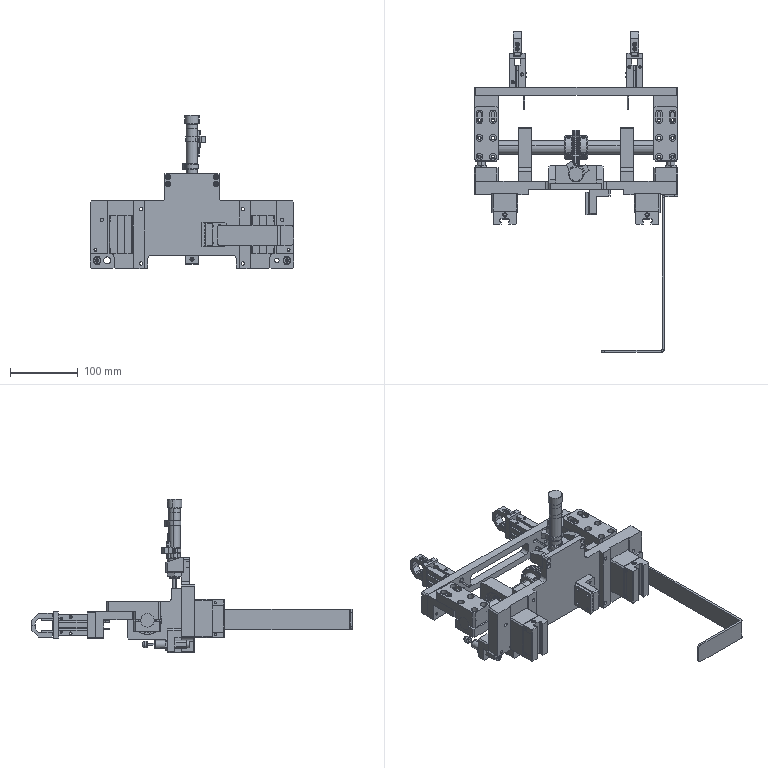Part | SolidWorks | features InContextFeatHolder 22, ReferencePattern 3, CompositeCurve 1, MirrorCompFeat 1 | 87 solids | 3073 faces | volume 1438864 mm3 | plane 1351 | cylinder 1242 | cone 308 | sphere 120 | torus 52 | commonest cylinder face diameters 0.5 x124 10 x82 4.2 x64 5.5 x56 29.9 x54 32.1 x54